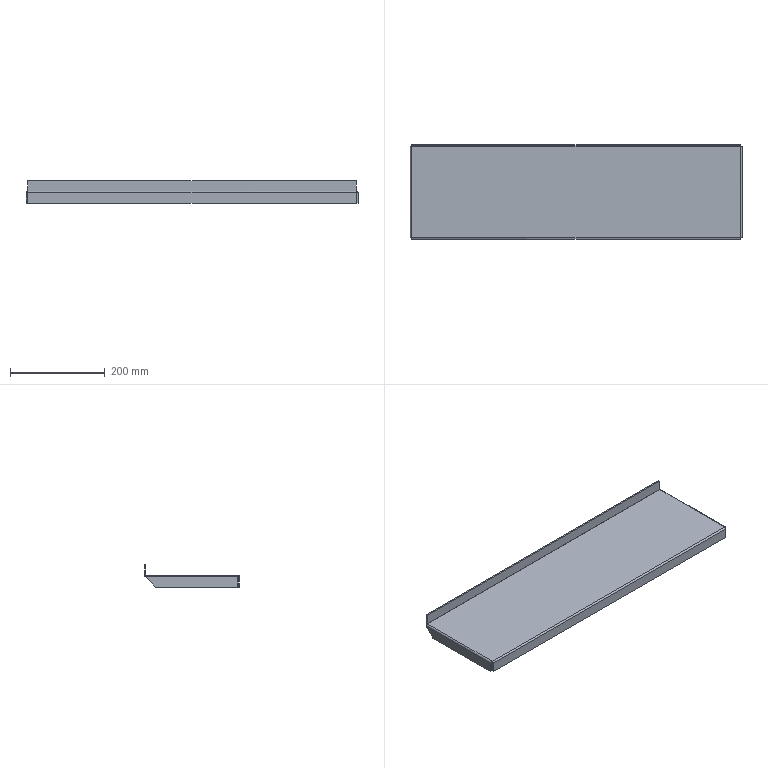Part | STEP file | PN_0017 304 stair tread_Default<As Machined> | 1 solid | 40 faces | box 700 x 200 x 47 mm | volume 531503 mm3 | plane 28 | cylinder 8 | spline 4 | commonest cylinder face diameters 0.6 x4 6.6 x4